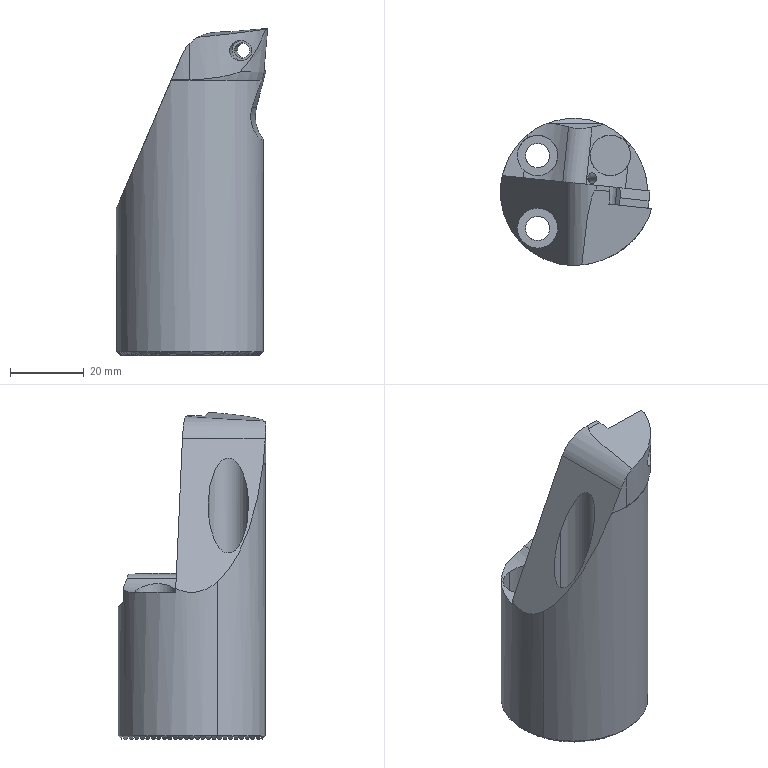NC program | Mastercam | posted with a generic post
Whole program:
%
:0001()
(MATERIAL - ALUMINUM MM - 2024)
(T10|50 FM/CTM |H10)
(T2|12 FEMR |H2|D2|WEAR COMP|TOOL DIA. - 12.|XY STOCK TO LEAVE - .3|Z STOCK TO LEAVE - 0.)
(T3|10 CHM |H3)
(T11|6.6 DR |H11)
(T7|3.3 DR |H7)
(T1|2.8 DR |H1)
(T16|6 FEM |H16|D16|WEAR COMP|TOOL DIA. - 6.)
(T4|11 DR |H4)
(T5|8 FEMR |H5|D5|WEAR COMP|TOOL DIA. - 8.|XY STOCK TO LEAVE - .05|Z STOCK TO LEAVE - .05)
(T6|8 FEMF |H6|D6|WEAR COMP|TOOL DIA. - 8.|XY STOCK TO LEAVE - .01|Z STOCK TO LEAVE - 0.)
(T14|5 DR |H14)
(T15|M6 X 1 RH |H15)
N100 G21
N102 G0 G17 G40 G80 G90 G94 G98
N104 G0 G28 G91 Z0.
N106 G0 G28 X0. Y0.
(50 FM/CTM |TOOL - 10|DIA. OFF. - 10|LEN. - 10|TOOL DIA. - 50.)
N108 T10 M6
N110 G0 G54 G90 X0. Y-55. C0. B0. S1600 M3
N112 G43 H10 Z53.5
N114 Z4.5
N116 G1 Z0. F600.
N118 Y-20.
N120 Y20.
N122 Y55.
N124 G0 Z53.5
N126 M5
N128 G0 G28 G91 Z0.
N130 G28
N132 M01
N134 G0 G17 G40 G80 G90 G94 G98
N136 G0 G28 G91 Z0.
(12 FEMR |TOOL - 2|DIA. OFF. - 2|LEN. - 2|TOOL DIA. - 12.)
N138 T2 M6
N140 G0 G54 G90 X-.747 Y35.706 C0. B0. S3500 M3
N142 G43 H2 Z50.
N144 Z1.
N146 G1 Z-1.5 F2000.
N148 G41 D2 X-.806 Y27.306 F400.
N150 Y27.299
N152 G3 X.187 Y26.299 I1.
N154 G2 X26.3 Y0. I-.187 J-26.299
N156 X0. Y-26.3 I-26.3
N158 X-26.3 Y0. J26.3
N160 X0. Y26.3 I26.3
N162 X.187 Y26.299 J-26.3
N164 X.687 Y26.291 I-.187 J-26.299
N166 G1 X.713
N168 G3 X1.712 Y27.265 J1.
N170 G1 G40 X1.932 Y35.662
N172 G0 Z50.
N174 M5
N176 G0 G28 G91 Z0.
N178 G28
N180 M01
N182 G0 G17 G40 G80 G90 G94 G98
N184 G0 G28 G91 Z0.
(10 CHM |TOOL - 3|DIA. OFF. - 3|LEN. - 3|TOOL DIA. - 10.)
N186 T3 M6
N188 G0 G54 G90 X9.899 Y-9.899 C0. B0. S2000 M3
N190 G43 H3 Z50.
N192 G81 G98 Z-3.8 R1. F100.
N194 Y9.899
N196 X-9.899
N198 G80
N200 M5
N202 G0 G28 G91 Z0.
N204 G28
N206 M01
N208 G0 G17 G40 G80 G90 G94 G98
N210 G0 G28 G91 Z0.
(6.6 DR |TOOL - 11|DIA. OFF. - 11|LEN. - 11|TOOL DIA. - 6.6)
N212 T11 M6
N214 G0 G54 G90 X-9.899 Y9.899 C0. B0. S2300 M3
N216 G43 H11 Z50.
N218 G81 G98 Z-9. R2. F60.
N220 X9.899
N222 Y-9.899
N224 G80
N226 M5
N228 G0 G28 G91 Z0.
N230 G28
N232 M01
N234 G0 G17 G40 G80 G90 G94 G98
N236 G0 G28 G91 Z0.
(3.3 DR |TOOL - 7|DIA. OFF. - 7|LEN. - 7|TOOL DIA. - 3.3)
N238 T7 M6
N240 G0 G54 G90 X0. Y3. C0. B0. S2300 M3
N242 G43 H7 Z50.
N244 G81 G98 Z-6. R2. F60.
N246 G80
N248 M5
N250 G0 G28 G91 Z0.
N252 G28
N254 M01
N256 G0 G17 G40 G80 G90 G94 G98
N258 G0 G28 G91 Z0.
(2.8 DR |TOOL - 1|DIA. OFF. - 1|LEN. - 1|TOOL DIA. - 2.8)
N260 T1 M6
N262 G0 G54 G90 X0. Y3. C0. B0. S2300 M3
N264 G43 H1 Z50.
N266 G83 G98 Z-28. R2. Q2. F30.
N268 G80
N270 M5
N272 G0 G28 G91 Z0.
N274 G28
N276 M01
N278 G0 G17 G40 G80 G90 G94 G98
N280 G0 G28 G91 Z0.
(6 FEM |TOOL - 16|DIA. OFF. - 16|LEN. - 16|TOOL DIA. - 6.)
N282 T16 M6
N284 G0 G54 G90 X0. Y.5 C0. B0. S4500 M3
N286 G43 H16 Z50.
N288 Z1.
N290 G1 Z0. F2000.
N292 G41 D16 X-2. F400.
N294 G3 X-2.5 Y0. J-.5
N296 X0. Y-2.5 Z-.075 I2.5
N298 X2.5 Y0. Z-.15 J2.5
N300 X0. Y2.5 Z-.225 I-2.5
N302 X-2.5 Y0. Z-.3 J-2.5
N304 X0. Y-2.5 Z-.375 I2.5
N306 X2.5 Y0. Z-.45 J2.5
N308 X0. Y2.5 Z-.525 I-2.5
N310 X-2.5 Y0. Z-.6 J-2.5
N312 X0. Y-2.5 Z-.675 I2.5
N314 X2.5 Y0. Z-.75 J2.5
N316 X0. Y2.5 Z-.825 I-2.5
N318 X-2.5 Y0. Z-.9 J-2.5
N320 X0. Y-2.5 Z-.975 I2.5
N322 X2.5 Y0. Z-1.05 J2.5
N324 X0. Y2.5 Z-1.125 I-2.5
N326 X-2.5 Y0. Z-1.2 J-2.5
N328 X0. Y-2.5 Z-1.275 I2.5
N330 X2.5 Y0. Z-1.35 J2.5
N332 X0. Y2.5 Z-1.425 I-2.5
N334 X-2.5 Y0. Z-1.5 J-2.5
N336 X0. Y-2.5 Z-1.575 I2.5
N338 X2.5 Y0. Z-1.65 J2.5
N340 X0. Y2.5 Z-1.725 I-2.5
N342 X-2.5 Y0. Z-1.8 J-2.5
N344 X0. Y-2.5 Z-1.875 I2.5
N346 X2.5 Y0. Z-1.95 J2.5
N348 X0. Y2.5 Z-2.025 I-2.5
N350 X-2.5 Y0. Z-2.1 J-2.5
N352 X0. Y-2.5 Z-2.175 I2.5
N354 X2.5 Y0. Z-2.25 J2.5
N356 X0. Y2.5 Z-2.325 I-2.5
N358 X-2.5 Y0. Z-2.4 J-2.5
N360 X0. Y-2.5 Z-2.475 I2.5
N362 X2.5 Y0. Z-2.55 J2.5
N364 X0. Y2.5 Z-2.625 I-2.5
N366 X-2.5 Y0. Z-2.7 J-2.5
N368 X0. Y-2.5 Z-2.775 I2.5
N370 X2.5 Y0. Z-2.85 J2.5
N372 X0. Y2.5 Z-2.925 I-2.5
N374 X-2.5 Y0. Z-3. J-2.5
N376 X0. Y-2.5 Z-3.075 I2.5
N378 X2.5 Y0. Z-3.15 J2.5
N380 X0. Y2.5 Z-3.225 I-2.5
N382 X-2.5 Y0. Z-3.3 J-2.5
N384 X0. Y-2.5 Z-3.375 I2.5
N386 X2.5 Y0. Z-3.45 J2.5
N388 X0. Y2.5 Z-3.525 I-2.5
N390 X-2.5 Y0. Z-3.6 J-2.5
N392 X0. Y-2.5 Z-3.675 I2.5
N394 X2.5 Y0. Z-3.75 J2.5
N396 X0. Y2.5 Z-3.825 I-2.5
N398 X-2.5 Y0. Z-3.9 J-2.5
N400 X0. Y-2.5 Z-3.975 I2.5
N402 X2.5 Y0. Z-4.05 J2.5
N404 X0. Y2.5 Z-4.125 I-2.5
N406 X-2.5 Y0. Z-4.2 J-2.5
N408 X0. Y-2.5 Z-4.275 I2.5
N410 X2.5 Y0. Z-4.35 J2.5
N412 X0. Y2.5 Z-4.425 I-2.5
N414 X-2.5 Y0. Z-4.5 J-2.5
N416 X0. Y-2.5 Z-4.575 I2.5
N418 X2.5 Y0. Z-4.65 J2.5
N420 X0. Y2.5 Z-4.725 I-2.5
N422 X-2.5 Y0. Z-4.8 J-2.5
N424 X0. Y-2.5 Z-4.875 I2.5
N426 X2.5 Y0. Z-4.95 J2.5
N428 X1.25 Y2.165 Z-5. I-2.5
N430 X0. Y2.5 I-1.25 J-2.165
N432 X-2.5 Y0. J-2.5
N434 X0. Y-2.5 I2.5
N436 X2.5 Y0. J2.5
N438 X.795 Y2.37 I-2.5
N440 X.636 Y2.396 I-.159 J-.474
N442 X.162 Y2.055 J-.5
N444 G1 G40 X-.474 Y.159
N446 G0 Z50.
N448 M5
N450 G0 G28 G91 Z0.
N452 G28
N454 M01
N456 G0 G17 G40 G80 G90 G94 G98
N458 G0 G28 G91 Z0.
(11 DR |TOOL - 4|DIA. OFF. - 4|LEN. - 4|TOOL DIA. - 11.)
N460 T4 M6
N462 G0 G54 G90 X0. Y0. C0. B0. S2000 M3
N464 G43 H4 Z50.
N466 G83 G98 Z-9.305 R1. Q4. F80.
N468 G80
N470 M5
N472 G0 G28 G91 Z0.
N474 G28
N476 M01
N478 G0 G17 G40 G80 G90 G94 G98
N480 G0 G28 G91 Z0.
(6 CBCHM |TOOL - 7|DIA. OFF. - 7|LEN. - 7|TOOL DIA. - 6.)
N482 T7 M6
N484 G0 G54 G90 X-.5 Y25.2 C0. B0. S3500 M3
N486 G43 H7 Z50.
N488 Z1.
N490 G1 Z-1.2 F2000.
N492 G41 D7 Y21. F400.
N494 G3 X0. Y20.5 I.5
N496 G2 X20.5 Y0. J-20.5
N498 X0. Y-20.5 I-20.5
N500 X-20.5 Y0. J20.5
N502 X0. Y20.5 I20.5
N504 X.5 Y20.494 J-20.5
N506 G1 X.512
N508 G3 X1.012 Y20.982 J.5
N510 G1 G40 X1.114 Y25.18
N512 G0 Z50.
N514 X2.529 Y.324
N516 Z1.
N518 G1 Z-1.8 F2000.
N520 G41 D7 X4.424 Y.963 F400.
N522 G3 X4.764 Y1.437 I-.16 J.474
N524 X4.738 Y1.596 I-.5
N526 X0. Y5. I-4.738 J-1.596
N528 X-5. Y0. J-5.
N530 X0. Y-5. I5.
N532 X5. Y0. J5.
N534 X4.738 Y1.596 I-5.
N536 X4.555 Y2.062 I-4.738 J-1.596
N538 X4.1 Y2.355 I-.455 J-.207
N540 X3.894 Y2.311 J-.5
N542 G1 G40 X2.071 Y1.486
N544 G0 Z50.
N546 M5
N548 G0 G28 G91 Z0.
N550 G28
N552 M01
N554 G0 G17 G40 G80 G90 G94 G98
N556 G0 G28 G91 Z0.
(8 FEMR |TOOL - 5|DIA. OFF. - 5|LEN. - 5|TOOL DIA. - 8.)
N558 T5 M6
N560 G0 G54 G90 X0. Y0. C0. B0. S3500 M3
N562 G43 H5 Z50.
N564 Z2.
N566 G1 Z-3.95 F2000.
N568 G41 D5 X-1.363 F400.
N570 G3 X-1.407 Y-.248 I.682 J-.248
N572 X-1.363 Y-.496 I.726
N574 X0. Y-1.45 I1.363 J.496
N576 X1.45 Y0. J1.45
N578 X0. Y1.45 I-1.45
N580 X-1.45 Y0. J-1.45
N582 X-1.363 Y-.496 I1.45
N584 X-1.311 Y-.619 I1.363 J.496
N586 X-.959 Y-.968 I.655 J.31
N588 G1 G40 X0. Y0.
N590 G41 D5 X-1.597
N592 G3 X-1.648 Y-.291 I.798 J-.291
N594 X-1.597 Y-.581 I.849
N596 X0. Y-1.699 I1.597 J.581
N598 X1.699 Y0. J1.699
N600 X0. Y1.699 I-1.699
N602 X-1.699 Y0. J-1.699
N604 X-1.597 Y-.581 I1.699
N606 X-1.54 Y-.719 I1.597 J.581
N608 X-1.129 Y-1.13 I.77 J.359
N610 G1 G40 X0. Y0.
N612 G41 D5 X-1.832
N614 G3 X-1.891 Y-.333 I.916 J-.333
N616 X-1.832 Y-.667 I.975
N618 X0. Y-1.95 I1.832 J.667
N620 X1.95 Y0. J1.95
N622 X0. Y1.95 I-1.95
N624 X-1.95 Y0. J-1.95
N626 X-1.832 Y-.667 I1.95
N628 X-1.77 Y-.818 I1.832 J.667
N630 X-1.3 Y-1.292 I.885 J.409
N632 G1 G40 X0. Y0.
N634 G0 Z50.
N636 M5
N638 G0 G28 G91 Z0.
N640 G28
N642 M01
N644 G0 G17 G40 G80 G90 G94 G98
N646 G0 G28 G91 Z0.
(8 FEMF |TOOL - 6|DIA. OFF. - 6|LEN. - 6|TOOL DIA. - 8.)
N648 T6 M6
N650 G0 G54 G90 X0. Y0. C0. B0. S3500 M3
N652 G43 H6 Z50.
N654 Z2.
N656 G1 Z-4. F2000.
N658 G41 D6 X-1.87 F400.
N660 G3 X-1.93 Y-.34 I.935 J-.34
N662 X-1.87 Y-.681 I.995
N664 X0. Y-1.99 I1.87 J.681
N666 X1.99 Y0. J1.99
N668 X0. Y1.99 I-1.99
N670 X-1.99 Y0. J-1.99
N672 X-1.87 Y-.681 I1.99
N674 X-1.807 Y-.834 I1.87 J.681
N676 X-1.327 Y-1.317 I.904 J.417
N678 G1 G40 X0. Y0.
N680 G41 D6 X-1.87
N682 G3 X-1.93 Y-.34 I.935 J-.34
N684 X-1.87 Y-.681 I.995
N686 X0. Y-1.99 I1.87 J.681
N688 X1.99 Y0. J1.99
N690 X0. Y1.99 I-1.99
N692 X-1.99 Y0. J-1.99
N694 X-1.87 Y-.681 I1.99
N696 X-1.807 Y-.834 I1.87 J.681
N698 X-1.327 Y-1.317 I.904 J.417
N700 G1 G40 X0. Y0.
N702 G41 D6 X-1.87
N704 G3 X-1.93 Y-.34 I.935 J-.34
N706 X-1.87 Y-.681 I.995
N708 X0. Y-1.99 I1.87 J.681
N710 X1.99 Y0. J1.99
N712 X0. Y1.99 I-1.99
N714 X-1.99 Y0. J-1.99
N716 X-1.87 Y-.681 I1.99
N718 X-1.807 Y-.834 I1.87 J.681
N720 X-1.327 Y-1.317 I.904 J.417
N722 G1 G40 X0. Y0.
N724 G0 Z50.
N726 M5
N728 G0 G28 G91 Z0.
N730 G28
N732 M01
N734 G0 G17 G40 G80 G90 G94 G98
N736 G0 G28 G91 Z0.
(5 DR |TOOL - 14|DIA. OFF. - 14|LEN. - 14|TOOL DIA. - 5.)
N738 M8
N740 T14 M6
N742 G0 G54 G90 X0. Y27.4 C0. B0. S3000 M3
N744 G43 H14 Z50.
N746 G83 G98 Z-20. R1. Q2. F300.
N748 X-23.729 Y-13.7
N750 X23.729
N752 G80
N754 M9
N756 M5
N758 G0 G28 G91 Z0.
N760 G28
N762 M01
N764 G0 G17 G40 G80 G90 G94 G98
N766 G0 G28 G91 Z0.
(M6 X 1 RH |TOOL - 15|DIA. OFF. - 15|LEN. - 15|TOOL DIA. - 6.)
N768 M8
N770 T15 M6
N772 G0 G54 G90 X0. Y27.4 C0. B0. S300 M3
N774 G43 H15 Z50.
N776 G84 G98 Z-10. R1. F300.
N778 X-23.729 Y-13.7
N780 X23.729
N782 G80
N784 M9
N786 M5
N788 G0 G28 G91 Z0.
N790 G0 G28 X0. Y0.
N792 G28
N794 M30
%